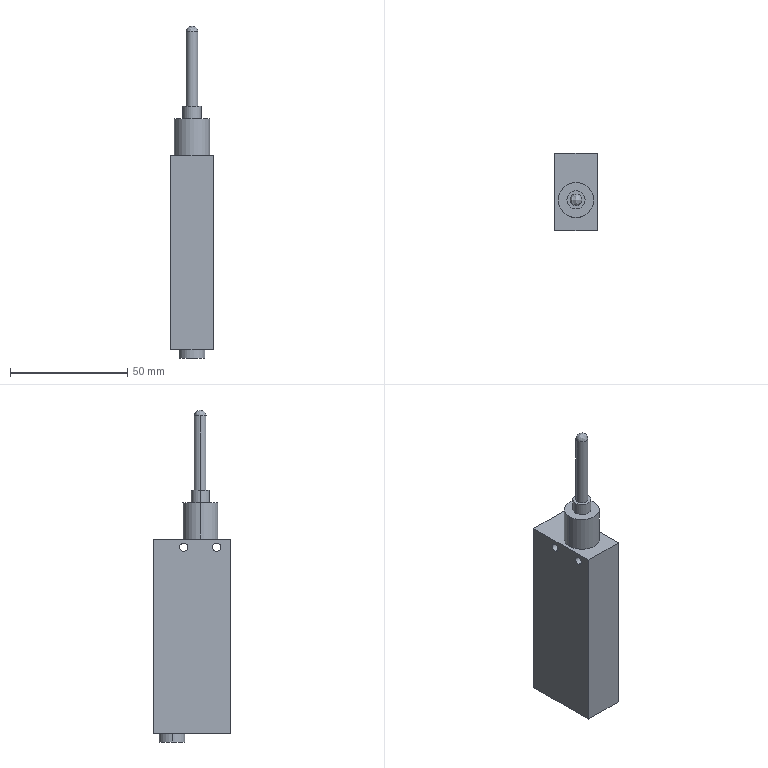Part | STEP file | GS-1713 (Ono) | 1 solid | 22 faces | box 18 x 33 x 141.5 mm | volume 52927 mm3 | cylinder 12 | plane 9 | spline 1 | commonest cylinder face diameters 3.5 x4 5 x2 7.7 x2 11 x2 15 x2